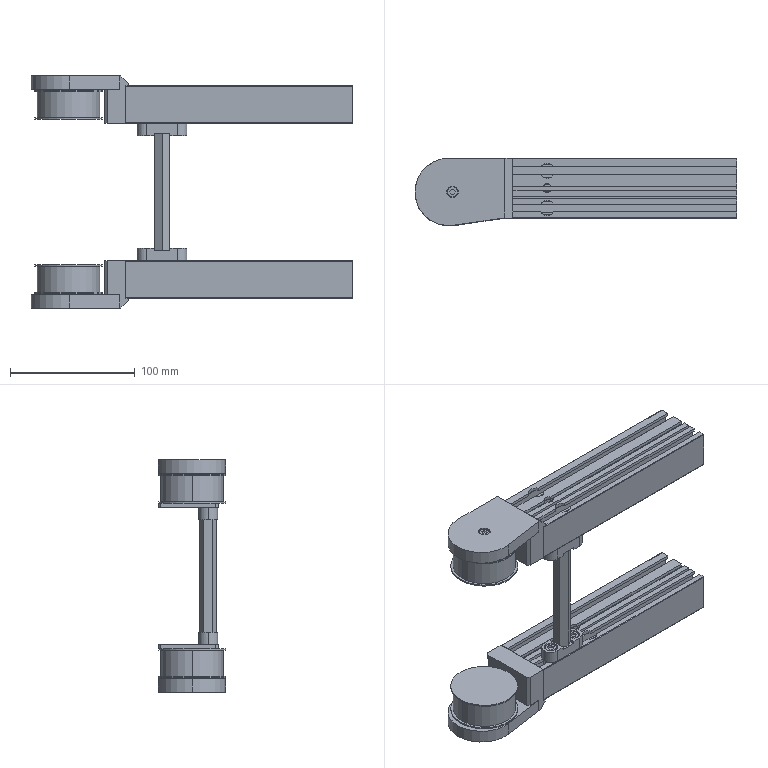Part | STEP file | Guide wheel mechanism revised.sldasm-Part-50 | 1 solid | 562 faces | box 258 x 54 x 186 mm | volume 573871 mm3 | plane 445 | cylinder 105 | cone 12 | commonest cylinder face diameters 12.2 x16 54 x11 1 x8 5 x8 6 x8 6.4 x8